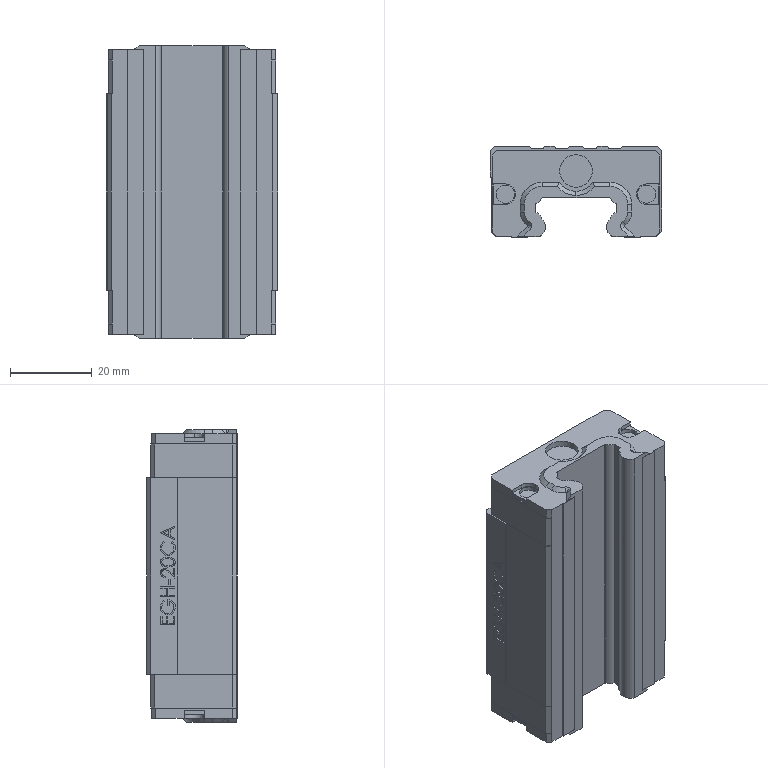Part | STEP file | EGH20CA Slider | 1 solid | 276 faces | box 42 x 22.2 x 71.7 mm | volume 50391 mm3 | plane 176 | cylinder 41 | spline 33 | cone 26 | commonest cylinder face diameters 4.2 x12 5 x9 2 x8 4.488 x4 8 x4 4.507 x2